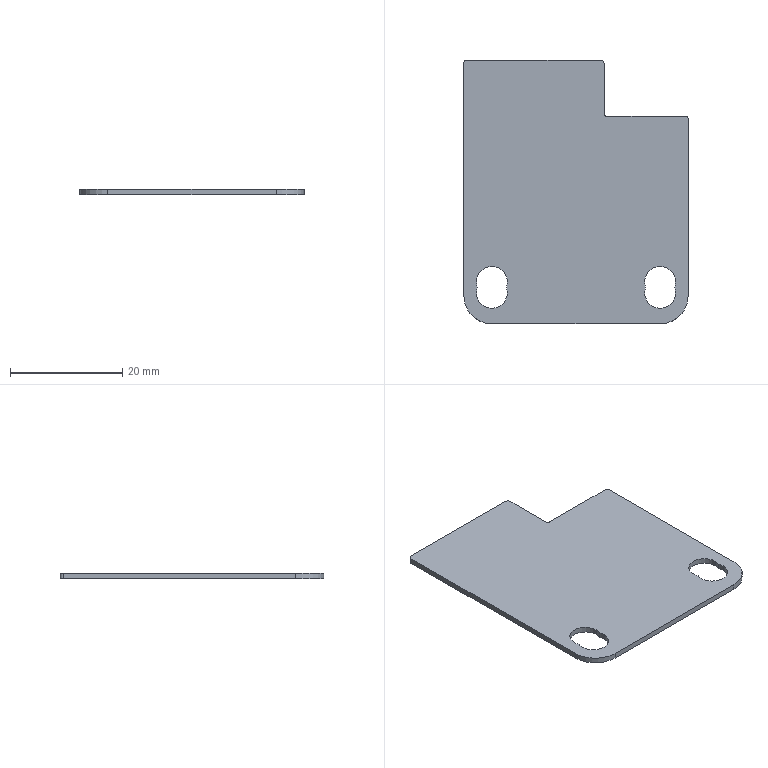Part | SolidWorks | features BaseBody 1 | 1 solid | 26 faces | box 40 x 47 x 1 mm | volume 1650 mm3 | cylinder 18 | plane 8 | commonest cylinder face diameters 5.5 x12 1 x4 10 x2
STEP:
#1=CARTESIAN_POINT('',(180.229,1870.544,-8.));
#2=VERTEX_POINT('',#1);
#3=CARTESIAN_POINT('',(180.041,1869.544,-8.));
#4=VERTEX_POINT('',#3);
#5=CARTESIAN_POINT('',(177.479,1870.544,-8.));
#6=DIRECTION('',(0.,0.,-1.));
#7=DIRECTION('',(-1.,0.,0.));
#8=AXIS2_PLACEMENT_3D('',#5,#6,#7);
#9=CIRCLE('',#8,2.75);
#10=EDGE_CURVE('',#2,#4,#9,.T.);
#11=ORIENTED_EDGE('',*,*,#10,.F.);
#12=CARTESIAN_POINT('',(180.229,1870.544,-9.));
#13=VERTEX_POINT('',#12);
#14=CARTESIAN_POINT('',(180.229,1870.544,-8.5));
#15=DIRECTION('',(0.,0.,-1.));
#16=VECTOR('',#15,1000.);
#17=LINE('',#14,#16);
#18=EDGE_CURVE('',#2,#13,#17,.T.);
#19=ORIENTED_EDGE('',*,*,#18,.T.);
#20=CARTESIAN_POINT('',(180.041,1869.544,-9.));
#21=VERTEX_POINT('',#20);
#22=CARTESIAN_POINT('',(177.479,1870.544,-9.));
#23=DIRECTION('',(0.,0.,1.));
#24=DIRECTION('',(-1.,0.,0.));
#25=AXIS2_PLACEMENT_3D('',#22,#23,#24);
#26=CIRCLE('',#25,2.75);
#27=EDGE_CURVE('',#21,#13,#26,.T.);
#28=ORIENTED_EDGE('',*,*,#27,.F.);
#29=CARTESIAN_POINT('',(180.041,1869.544,-8.5));
#30=DIRECTION('',(0.,0.,-1.));
#31=VECTOR('',#30,1000.);
#32=LINE('',#29,#31);
#33=EDGE_CURVE('',#4,#21,#32,.T.);
#34=ORIENTED_EDGE('',*,*,#33,.F.);
#35=EDGE_LOOP('',(#11,#19,#28,#34));
#36=FACE_OUTER_BOUND('',#35,.T.);
#37=CARTESIAN_POINT('',(177.479,1870.544,-8.5));
#38=DIRECTION('',(0.,0.,-1.));
#39=DIRECTION('',(-1.,0.,0.));
#40=AXIS2_PLACEMENT_3D('',#37,#38,#39);
#41=CYLINDRICAL_SURFACE('',#40,2.75);
#42=ADVANCED_FACE('',(#36),#41,.F.);
#43=ORIENTED_EDGE('',*,*,#18,.F.);
#44=CARTESIAN_POINT('',(174.729,1870.544,-8.));
#45=VERTEX_POINT('',#44);
#46=CARTESIAN_POINT('',(177.479,1870.544,-8.));
#47=DIRECTION('',(0.,0.,-1.));
#48=DIRECTION('',(-1.,0.,0.));
#49=AXIS2_PLACEMENT_3D('',#46,#47,#48);
#50=CIRCLE('',#49,2.75);
#51=EDGE_CURVE('',#45,#2,#50,.T.);
#52=ORIENTED_EDGE('',*,*,#51,.F.);
#53=CARTESIAN_POINT('',(174.729,1870.544,-9.));
#54=VERTEX_POINT('',#53);
#55=CARTESIAN_POINT('',(174.729,1870.544,-8.5));
#56=DIRECTION('',(0.,0.,-1.));
#57=VECTOR('',#56,1000.);
#58=LINE('',#55,#57);
#59=EDGE_CURVE('',#45,#54,#58,.T.);
#60=ORIENTED_EDGE('',*,*,#59,.T.);
#61=CARTESIAN_POINT('',(177.479,1870.544,-9.));
#62=DIRECTION('',(0.,0.,1.));
#63=DIRECTION('',(-1.,0.,0.));
#64=AXIS2_PLACEMENT_3D('',#61,#62,#63);
#65=CIRCLE('',#64,2.75);
#66=EDGE_CURVE('',#13,#54,#65,.T.);
#67=ORIENTED_EDGE('',*,*,#66,.F.);
#68=EDGE_LOOP('',(#43,#52,#60,#67));
#69=FACE_OUTER_BOUND('',#68,.T.);
#70=CARTESIAN_POINT('',(177.479,1870.544,-8.5));
#71=DIRECTION('',(0.,0.,-1.));
#72=DIRECTION('',(-1.,0.,0.));
#73=AXIS2_PLACEMENT_3D('',#70,#71,#72);
#74=CYLINDRICAL_SURFACE('',#73,2.75);
#75=ADVANCED_FACE('',(#69),#74,.F.);
#76=CARTESIAN_POINT('',(180.229,1868.544,-8.));
#77=VERTEX_POINT('',#76);
#78=CARTESIAN_POINT('',(174.729,1868.544,-8.));
#79=VERTEX_POINT('',#78);
#80=CARTESIAN_POINT('',(177.479,1868.544,-8.));
#81=DIRECTION('',(0.,0.,-1.));
#82=DIRECTION('',(-1.,0.,0.));
#83=AXIS2_PLACEMENT_3D('',#80,#81,#82);
#84=CIRCLE('',#83,2.75);
#85=EDGE_CURVE('',#77,#79,#84,.T.);
#86=ORIENTED_EDGE('',*,*,#85,.F.);
#87=CARTESIAN_POINT('',(180.229,1868.544,-9.));
#88=VERTEX_POINT('',#87);
#89=CARTESIAN_POINT('',(180.229,1868.544,-8.5));
#90=DIRECTION('',(0.,0.,-1.));
#91=VECTOR('',#90,1000.);
#92=LINE('',#89,#91);
#93=EDGE_CURVE('',#77,#88,#92,.T.);
#94=ORIENTED_EDGE('',*,*,#93,.T.);
#95=CARTESIAN_POINT('',(174.729,1868.544,-9.));
#96=VERTEX_POINT('',#95);
#97=CARTESIAN_POINT('',(177.479,1868.544,-9.));
#98=DIRECTION('',(0.,0.,1.));
#99=DIRECTION('',(-1.,0.,0.));
#100=AXIS2_PLACEMENT_3D('',#97,#98,#99);
#101=CIRCLE('',#100,2.75);
#102=EDGE_CURVE('',#96,#88,#101,.T.);
#103=ORIENTED_EDGE('',*,*,#102,.F.);
#104=CARTESIAN_POINT('',(174.729,1868.544,-8.5));
#105=DIRECTION('',(0.,0.,-1.));
#106=VECTOR('',#105,1000.);
#107=LINE('',#104,#106);
#108=EDGE_CURVE('',#79,#96,#107,.T.);
#109=ORIENTED_EDGE('',*,*,#108,.F.);
#110=EDGE_LOOP('',(#86,#94,#103,#109));
#111=FACE_OUTER_BOUND('',#110,.T.);
#112=CARTESIAN_POINT('',(177.479,1868.544,-8.5));
#113=DIRECTION('',(0.,0.,-1.));
#114=DIRECTION('',(-1.,0.,0.));
#115=AXIS2_PLACEMENT_3D('',#112,#113,#114);
#116=CYLINDRICAL_SURFACE('',#115,2.75);
#117=ADVANCED_FACE('',(#111),#116,.F.);
#118=CARTESIAN_POINT('',(174.917,1869.544,-8.));
#119=VERTEX_POINT('',#118);
#120=CARTESIAN_POINT('',(177.479,1868.544,-8.));
#121=DIRECTION('',(0.,0.,-1.));
#122=DIRECTION('',(-1.,0.,0.));
#123=AXIS2_PLACEMENT_3D('',#120,#121,#122);
#124=CIRCLE('',#123,2.75);
#125=EDGE_CURVE('',#79,#119,#124,.T.);
#126=ORIENTED_EDGE('',*,*,#125,.F.);
#127=ORIENTED_EDGE('',*,*,#108,.T.);
#128=CARTESIAN_POINT('',(174.917,1869.544,-9.));
#129=VERTEX_POINT('',#128);
#130=CARTESIAN_POINT('',(177.479,1868.544,-9.));
#131=DIRECTION('',(0.,0.,1.));
#132=DIRECTION('',(-1.,0.,0.));
#133=AXIS2_PLACEMENT_3D('',#130,#131,#132);
#134=CIRCLE('',#133,2.75);
#135=EDGE_CURVE('',#129,#96,#134,.T.);
#136=ORIENTED_EDGE('',*,*,#135,.F.);
#137=CARTESIAN_POINT('',(174.917,1869.544,-8.5));
#138=DIRECTION('',(0.,0.,1.));
#139=VECTOR('',#138,1000.);
#140=LINE('',#137,#139);
#141=EDGE_CURVE('',#129,#119,#140,.T.);
#142=ORIENTED_EDGE('',*,*,#141,.T.);
#143=EDGE_LOOP('',(#126,#127,#136,#142));
#144=FACE_OUTER_BOUND('',#143,.T.);
#145=CARTESIAN_POINT('',(177.479,1868.544,-8.5));
#146=DIRECTION('',(0.,0.,-1.));
#147=DIRECTION('',(-1.,0.,0.));
#148=AXIS2_PLACEMENT_3D('',#145,#146,#147);
#149=CYLINDRICAL_SURFACE('',#148,2.75);
#150=ADVANCED_FACE('',(#144),#149,.F.);
#151=CARTESIAN_POINT('',(204.729,1870.544,-9.));
#152=VERTEX_POINT('',#151);
#153=CARTESIAN_POINT('',(204.917,1869.544,-9.));
#154=VERTEX_POINT('',#153);
#155=CARTESIAN_POINT('',(207.479,1870.544,-9.));
#156=DIRECTION('',(0.,0.,1.));
#157=DIRECTION('',(1.,0.,0.));
#158=AXIS2_PLACEMENT_3D('',#155,#156,#157);
#159=CIRCLE('',#158,2.75);
#160=EDGE_CURVE('',#152,#154,#159,.T.);
#161=ORIENTED_EDGE('',*,*,#160,.F.);
#162=CARTESIAN_POINT('',(204.729,1870.544,-8.));
#163=VERTEX_POINT('',#162);
#164=CARTESIAN_POINT('',(204.729,1870.544,-8.5));
#165=DIRECTION('',(0.,0.,1.));
#166=VECTOR('',#165,1000.);
#167=LINE('',#164,#166);
#168=EDGE_CURVE('',#152,#163,#167,.T.);
#169=ORIENTED_EDGE('',*,*,#168,.T.);
#170=CARTESIAN_POINT('',(204.917,1869.544,-8.));
#171=VERTEX_POINT('',#170);
#172=CARTESIAN_POINT('',(207.479,1870.544,-8.));
#173=DIRECTION('',(0.,0.,-1.));
#174=DIRECTION('',(1.,0.,0.));
#175=AXIS2_PLACEMENT_3D('',#172,#173,#174);
#176=CIRCLE('',#175,2.75);
#177=EDGE_CURVE('',#171,#163,#176,.T.);
#178=ORIENTED_EDGE('',*,*,#177,.F.);
#179=CARTESIAN_POINT('',(204.917,1869.544,-8.5));
#180=DIRECTION('',(0.,0.,1.));
#181=VECTOR('',#180,1000.);
#182=LINE('',#179,#181);
#183=EDGE_CURVE('',#154,#171,#182,.T.);
#184=ORIENTED_EDGE('',*,*,#183,.F.);
#185=EDGE_LOOP('',(#161,#169,#178,#184));
#186=FACE_OUTER_BOUND('',#185,.T.);
#187=CARTESIAN_POINT('',(207.479,1870.544,-8.5));
#188=DIRECTION('',(0.,0.,1.));
#189=DIRECTION('',(1.,0.,0.));
#190=AXIS2_PLACEMENT_3D('',#187,#188,#189);
#191=CYLINDRICAL_SURFACE('',#190,2.75);
#192=ADVANCED_FACE('',(#186),#191,.F.);
#193=ORIENTED_EDGE('',*,*,#168,.F.);
#194=CARTESIAN_POINT('',(210.229,1870.544,-9.));
#195=VERTEX_POINT('',#194);
#196=CARTESIAN_POINT('',(207.479,1870.544,-9.));
#197=DIRECTION('',(0.,0.,1.));
#198=DIRECTION('',(1.,0.,0.));
#199=AXIS2_PLACEMENT_3D('',#196,#197,#198);
#200=CIRCLE('',#199,2.75);
#201=EDGE_CURVE('',#195,#152,#200,.T.);
#202=ORIENTED_EDGE('',*,*,#201,.F.);
#203=CARTESIAN_POINT('',(210.229,1870.544,-8.));
#204=VERTEX_POINT('',#203);
#205=CARTESIAN_POINT('',(210.229,1870.544,-8.5));
#206=DIRECTION('',(0.,0.,1.));
#207=VECTOR('',#206,1000.);
#208=LINE('',#205,#207);
#209=EDGE_CURVE('',#195,#204,#208,.T.);
#210=ORIENTED_EDGE('',*,*,#209,.T.);
#211=CARTESIAN_POINT('',(207.479,1870.544,-8.));
#212=DIRECTION('',(0.,0.,-1.));
#213=DIRECTION('',(1.,0.,0.));
#214=AXIS2_PLACEMENT_3D('',#211,#212,#213);
#215=CIRCLE('',#214,2.75);
#216=EDGE_CURVE('',#163,#204,#215,.T.);
#217=ORIENTED_EDGE('',*,*,#216,.F.);
#218=EDGE_LOOP('',(#193,#202,#210,#217));
#219=FACE_OUTER_BOUND('',#218,.T.);
#220=CARTESIAN_POINT('',(207.479,1870.544,-8.5));
#221=DIRECTION('',(0.,0.,1.));
#222=DIRECTION('',(1.,0.,0.));
#223=AXIS2_PLACEMENT_3D('',#220,#221,#222);
#224=CYLINDRICAL_SURFACE('',#223,2.75);
#225=ADVANCED_FACE('',(#219),#224,.F.);
#226=CARTESIAN_POINT('',(204.729,1868.544,-9.));
#227=VERTEX_POINT('',#226);
#228=CARTESIAN_POINT('',(210.229,1868.544,-9.));
#229=VERTEX_POINT('',#228);
#230=CARTESIAN_POINT('',(207.479,1868.544,-9.));
#231=DIRECTION('',(0.,0.,1.));
#232=DIRECTION('',(1.,0.,0.));
#233=AXIS2_PLACEMENT_3D('',#230,#231,#232);
#234=CIRCLE('',#233,2.75);
#235=EDGE_CURVE('',#227,#229,#234,.T.);
#236=ORIENTED_EDGE('',*,*,#235,.F.);
#237=CARTESIAN_POINT('',(204.729,1868.544,-8.));
#238=VERTEX_POINT('',#237);
#239=CARTESIAN_POINT('',(204.729,1868.544,-8.5));
#240=DIRECTION('',(0.,0.,1.));
#241=VECTOR('',#240,1000.);
#242=LINE('',#239,#241);
#243=EDGE_CURVE('',#227,#238,#242,.T.);
#244=ORIENTED_EDGE('',*,*,#243,.T.);
#245=CARTESIAN_POINT('',(210.229,1868.544,-8.));
#246=VERTEX_POINT('',#245);
#247=CARTESIAN_POINT('',(207.479,1868.544,-8.));
#248=DIRECTION('',(0.,0.,-1.));
#249=DIRECTION('',(1.,0.,0.));
#250=AXIS2_PLACEMENT_3D('',#247,#248,#249);
#251=CIRCLE('',#250,2.75);
#252=EDGE_CURVE('',#246,#238,#251,.T.);
#253=ORIENTED_EDGE('',*,*,#252,.F.);
#254=CARTESIAN_POINT('',(210.229,1868.544,-8.5));
#255=DIRECTION('',(0.,0.,1.));
#256=VECTOR('',#255,1000.);
#257=LINE('',#254,#256);
#258=EDGE_CURVE('',#229,#246,#257,.T.);
#259=ORIENTED_EDGE('',*,*,#258,.F.);
#260=EDGE_LOOP('',(#236,#244,#253,#259));
#261=FACE_OUTER_BOUND('',#260,.T.);
#262=CARTESIAN_POINT('',(207.479,1868.544,-8.5));
#263=DIRECTION('',(0.,0.,1.));
#264=DIRECTION('',(1.,0.,0.));
#265=AXIS2_PLACEMENT_3D('',#262,#263,#264);
#266=CYLINDRICAL_SURFACE('',#265,2.75);
#267=ADVANCED_FACE('',(#261),#266,.F.);
#268=CARTESIAN_POINT('',(210.041,1869.544,-9.));
#269=VERTEX_POINT('',#268);
#270=CARTESIAN_POINT('',(207.479,1868.544,-9.));
#271=DIRECTION('',(0.,0.,1.));
#272=DIRECTION('',(1.,0.,0.));
#273=AXIS2_PLACEMENT_3D('',#270,#271,#272);
#274=CIRCLE('',#273,2.75);
#275=EDGE_CURVE('',#229,#269,#274,.T.);
#276=ORIENTED_EDGE('',*,*,#275,.F.);
#277=ORIENTED_EDGE('',*,*,#258,.T.);
#278=CARTESIAN_POINT('',(210.041,1869.544,-8.));
#279=VERTEX_POINT('',#278);
#280=CARTESIAN_POINT('',(207.479,1868.544,-8.));
#281=DIRECTION('',(0.,0.,-1.));
#282=DIRECTION('',(1.,0.,0.));
#283=AXIS2_PLACEMENT_3D('',#280,#281,#282);
#284=CIRCLE('',#283,2.75);
#285=EDGE_CURVE('',#279,#246,#284,.T.);
#286=ORIENTED_EDGE('',*,*,#285,.F.);
#287=CARTESIAN_POINT('',(210.041,1869.544,-8.5));
#288=DIRECTION('',(0.,0.,-1.));
#289=VECTOR('',#288,1000.);
#290=LINE('',#287,#289);
#291=EDGE_CURVE('',#279,#269,#290,.T.);
#292=ORIENTED_EDGE('',*,*,#291,.T.);
#293=EDGE_LOOP('',(#276,#277,#286,#292));
#294=FACE_OUTER_BOUND('',#293,.T.);
#295=CARTESIAN_POINT('',(207.479,1868.544,-8.5));
#296=DIRECTION('',(0.,0.,1.));
#297=DIRECTION('',(1.,0.,0.));
#298=AXIS2_PLACEMENT_3D('',#295,#296,#297);
#299=CYLINDRICAL_SURFACE('',#298,2.75);
#300=ADVANCED_FACE('',(#294),#299,.F.);
#301=CARTESIAN_POINT('',(177.479,1868.544,-8.));
#302=DIRECTION('',(0.,0.,-1.));
#303=DIRECTION('',(-1.,0.,0.));
#304=AXIS2_PLACEMENT_3D('',#301,#302,#303);
#305=CIRCLE('',#304,2.75);
#306=EDGE_CURVE('',#4,#77,#305,.T.);
#307=ORIENTED_EDGE('',*,*,#306,.T.);
#308=ORIENTED_EDGE('',*,*,#85,.T.);
#309=ORIENTED_EDGE('',*,*,#125,.T.);
#310=CARTESIAN_POINT('',(177.479,1870.544,-8.));
#311=DIRECTION('',(0.,0.,-1.));
#312=DIRECTION('',(-1.,0.,0.));
#313=AXIS2_PLACEMENT_3D('',#310,#311,#312);
#314=CIRCLE('',#313,2.75);
#315=EDGE_CURVE('',#119,#45,#314,.T.);
#316=ORIENTED_EDGE('',*,*,#315,.T.);
#317=ORIENTED_EDGE('',*,*,#51,.T.);
#318=ORIENTED_EDGE('',*,*,#10,.T.);
#319=EDGE_LOOP('',(#307,#308,#309,#316,#317,#318));
#320=FACE_BOUND('',#319,.T.);
#321=ORIENTED_EDGE('',*,*,#285,.T.);
#322=ORIENTED_EDGE('',*,*,#252,.T.);
#323=CARTESIAN_POINT('',(207.479,1868.544,-8.));
#324=DIRECTION('',(0.,0.,-1.));
#325=DIRECTION('',(1.,0.,0.));
#326=AXIS2_PLACEMENT_3D('',#323,#324,#325);
#327=CIRCLE('',#326,2.75);
#328=EDGE_CURVE('',#238,#171,#327,.T.);
#329=ORIENTED_EDGE('',*,*,#328,.T.);
#330=ORIENTED_EDGE('',*,*,#177,.T.);
#331=ORIENTED_EDGE('',*,*,#216,.T.);
#332=CARTESIAN_POINT('',(207.479,1870.544,-8.));
#333=DIRECTION('',(0.,0.,-1.));
#334=DIRECTION('',(1.,0.,0.));
#335=AXIS2_PLACEMENT_3D('',#332,#333,#334);
#336=CIRCLE('',#335,2.75);
#337=EDGE_CURVE('',#204,#279,#336,.T.);
#338=ORIENTED_EDGE('',*,*,#337,.T.);
#339=EDGE_LOOP('',(#321,#322,#329,#330,#331,#338));
#340=FACE_BOUND('',#339,.T.);
#341=CARTESIAN_POINT('',(211.979,1900.044,-8.));
#342=VERTEX_POINT('',#341);
#343=CARTESIAN_POINT('',(197.979,1900.044,-8.));
#344=VERTEX_POINT('',#343);
#345=CARTESIAN_POINT('',(192.479,1900.044,-8.));
#346=DIRECTION('',(-1.,0.,0.));
#347=VECTOR('',#346,1000.);
#348=LINE('',#345,#347);
#349=EDGE_CURVE('',#342,#344,#348,.T.);
#350=ORIENTED_EDGE('',*,*,#349,.T.);
#351=CARTESIAN_POINT('',(197.479,1900.544,-8.));
#352=VERTEX_POINT('',#351);
#353=CARTESIAN_POINT('',(197.979,1900.544,-8.));
#354=DIRECTION('',(0.,0.,-1.));
#355=DIRECTION('',(-1.,0.,0.));
#356=AXIS2_PLACEMENT_3D('',#353,#354,#355);
#357=CIRCLE('',#356,0.5);
#358=EDGE_CURVE('',#344,#352,#357,.T.);
#359=ORIENTED_EDGE('',*,*,#358,.T.);
#360=CARTESIAN_POINT('',(197.479,1909.544,-8.));
#361=VERTEX_POINT('',#360);
#362=CARTESIAN_POINT('',(197.479,1886.544,-8.));
#363=DIRECTION('',(0.,1.,0.));
#364=VECTOR('',#363,1000.);
#365=LINE('',#362,#364);
#366=EDGE_CURVE('',#352,#361,#365,.T.);
#367=ORIENTED_EDGE('',*,*,#366,.T.);
#368=CARTESIAN_POINT('',(196.979,1910.044,-8.));
#369=VERTEX_POINT('',#368);
#370=CARTESIAN_POINT('',(196.979,1909.544,-8.));
#371=DIRECTION('',(0.,0.,1.));
#372=DIRECTION('',(-1.,0.,0.));
#373=AXIS2_PLACEMENT_3D('',#370,#371,#372);
#374=CIRCLE('',#373,0.5);
#375=EDGE_CURVE('',#361,#369,#374,.T.);
#376=ORIENTED_EDGE('',*,*,#375,.T.);
#377=CARTESIAN_POINT('',(172.979,1910.044,-8.));
#378=VERTEX_POINT('',#377);
#379=CARTESIAN_POINT('',(192.479,1910.044,-8.));
#380=DIRECTION('',(-1.,0.,0.));
#381=VECTOR('',#380,1000.);
#382=LINE('',#379,#381);
#383=EDGE_CURVE('',#369,#378,#382,.T.);
#384=ORIENTED_EDGE('',*,*,#383,.T.);
#385=CARTESIAN_POINT('',(172.479,1909.544,-8.));
#386=VERTEX_POINT('',#385);
#387=CARTESIAN_POINT('',(172.979,1909.544,-8.));
#388=DIRECTION('',(0.,0.,1.));
#389=DIRECTION('',(1.,0.,0.));
#390=AXIS2_PLACEMENT_3D('',#387,#388,#389);
#391=CIRCLE('',#390,0.5);
#392=EDGE_CURVE('',#378,#386,#391,.T.);
#393=ORIENTED_EDGE('',*,*,#392,.T.);
#394=CARTESIAN_POINT('',(172.479,1868.044,-8.));
#395=VERTEX_POINT('',#394);
#396=CARTESIAN_POINT('',(172.479,1886.544,-8.));
#397=DIRECTION('',(0.,-1.,0.));
#398=VECTOR('',#397,1000.);
#399=LINE('',#396,#398);
#400=EDGE_CURVE('',#386,#395,#399,.T.);
#401=ORIENTED_EDGE('',*,*,#400,.T.);
#402=CARTESIAN_POINT('',(177.479,1863.044,-8.));
#403=VERTEX_POINT('',#402);
#404=CARTESIAN_POINT('',(177.479,1868.044,-8.));
#405=DIRECTION('',(0.,0.,1.));
#406=DIRECTION('',(1.,0.,0.));
#407=AXIS2_PLACEMENT_3D('',#404,#405,#406);
#408=CIRCLE('',#407,5.);
#409=EDGE_CURVE('',#395,#403,#408,.T.);
#410=ORIENTED_EDGE('',*,*,#409,.T.);
#411=CARTESIAN_POINT('',(207.479,1863.044,-8.));
#412=VERTEX_POINT('',#411);
#413=CARTESIAN_POINT('',(192.479,1863.044,-8.));
#414=DIRECTION('',(1.,0.,0.));
#415=VECTOR('',#414,1000.);
#416=LINE('',#413,#415);
#417=EDGE_CURVE('',#403,#412,#416,.T.);
#418=ORIENTED_EDGE('',*,*,#417,.T.);
#419=CARTESIAN_POINT('',(212.479,1868.044,-8.));
#420=VERTEX_POINT('',#419);
#421=CARTESIAN_POINT('',(207.479,1868.044,-8.));
#422=DIRECTION('',(0.,0.,1.));
#423=DIRECTION('',(1.,0.,0.));
#424=AXIS2_PLACEMENT_3D('',#421,#422,#423);
#425=CIRCLE('',#424,5.);
#426=EDGE_CURVE('',#412,#420,#425,.T.);
#427=ORIENTED_EDGE('',*,*,#426,.T.);
#428=CARTESIAN_POINT('',(212.479,1899.544,-8.));
#429=VERTEX_POINT('',#428);
#430=CARTESIAN_POINT('',(212.479,1886.544,-8.));
#431=DIRECTION('',(0.,1.,0.));
#432=VECTOR('',#431,1000.);
#433=LINE('',#430,#432);
#434=EDGE_CURVE('',#420,#429,#433,.T.);
#435=ORIENTED_EDGE('',*,*,#434,.T.);
#436=CARTESIAN_POINT('',(211.979,1899.544,-8.));
#437=DIRECTION('',(0.,0.,1.));
#438=DIRECTION('',(1.,0.,0.));
#439=AXIS2_PLACEMENT_3D('',#436,#437,#438);
#440=CIRCLE('',#439,0.5);
#441=EDGE_CURVE('',#429,#342,#440,.T.);
#442=ORIENTED_EDGE('',*,*,#441,.T.);
#443=EDGE_LOOP('',(#350,#359,#367,#376,#384,#393,#401,#410,#418,#427,#435,#442));
#444=FACE_OUTER_BOUND('',#443,.T.);
#445=CARTESIAN_POINT('',(192.479,1886.544,-8.));
#446=DIRECTION('',(0.,0.,1.));
#447=DIRECTION('',(1.,0.,0.));
#448=AXIS2_PLACEMENT_3D('',#445,#446,#447);
#449=PLANE('',#448);
#450=ADVANCED_FACE('',(#320,#340,#444),#449,.T.);
#451=ORIENTED_EDGE('',*,*,#59,.F.);
#452=ORIENTED_EDGE('',*,*,#315,.F.);
#453=ORIENTED_EDGE('',*,*,#141,.F.);
#454=CARTESIAN_POINT('',(177.479,1870.544,-9.));
#455=DIRECTION('',(0.,0.,1.));
#456=DIRECTION('',(-1.,0.,0.));
#457=AXIS2_PLACEMENT_3D('',#454,#455,#456);
#458=CIRCLE('',#457,2.75);
#459=EDGE_CURVE('',#54,#129,#458,.T.);
#460=ORIENTED_EDGE('',*,*,#459,.F.);
#461=EDGE_LOOP('',(#451,#452,#453,#460));
#462=FACE_OUTER_BOUND('',#461,.T.);
#463=CARTESIAN_POINT('',(177.479,1870.544,-8.5));
#464=DIRECTION('',(0.,0.,-1.));
#465=DIRECTION('',(-1.,0.,0.));
#466=AXIS2_PLACEMENT_3D('',#463,#464,#465);
#467=CYLINDRICAL_SURFACE('',#466,2.75);
#468=ADVANCED_FACE('',(#462),#467,.F.);
#469=ORIENTED_EDGE('',*,*,#93,.F.);
#470=ORIENTED_EDGE('',*,*,#306,.F.);
#471=ORIENTED_EDGE('',*,*,#33,.T.);
#472=CARTESIAN_POINT('',(177.479,1868.544,-9.));
#473=DIRECTION('',(0.,0.,1.));
#474=DIRECTION('',(-1.,0.,0.));
#475=AXIS2_PLACEMENT_3D('',#472,#473,#474);
#476=CIRCLE('',#475,2.75);
#477=EDGE_CURVE('',#88,#21,#476,.T.);
#478=ORIENTED_EDGE('',*,*,#477,.F.);
#479=EDGE_LOOP('',(#469,#470,#471,#478));
#480=FACE_OUTER_BOUND('',#479,.T.);
#481=CARTESIAN_POINT('',(177.479,1868.544,-8.5));
#482=DIRECTION('',(0.,0.,-1.));
#483=DIRECTION('',(-1.,0.,0.));
#484=AXIS2_PLACEMENT_3D('',#481,#482,#483);
#485=CYLINDRICAL_SURFACE('',#484,2.75);
#486=ADVANCED_FACE('',(#480),#485,.F.);
#487=ORIENTED_EDGE('',*,*,#209,.F.);
#488=CARTESIAN_POINT('',(207.479,1870.544,-9.));
#489=DIRECTION('',(0.,0.,1.));
#490=DIRECTION('',(1.,0.,0.));
#491=AXIS2_PLACEMENT_3D('',#488,#489,#490);
#492=CIRCLE('',#491,2.75);
#493=EDGE_CURVE('',#269,#195,#492,.T.);
#494=ORIENTED_EDGE('',*,*,#493,.F.);
#495=ORIENTED_EDGE('',*,*,#291,.F.);
#496=ORIENTED_EDGE('',*,*,#337,.F.);
#497=EDGE_LOOP('',(#487,#494,#495,#496));
#498=FACE_OUTER_BOUND('',#497,.T.);
#499=CARTESIAN_POINT('',(207.479,1870.544,-8.5));
#500=DIRECTION('',(0.,0.,1.));
#501=DIRECTION('',(1.,0.,0.));
#502=AXIS2_PLACEMENT_3D('',#499,#500,#501);
#503=CYLINDRICAL_SURFACE('',#502,2.75);
#504=ADVANCED_FACE('',(#498),#503,.F.);
#505=ORIENTED_EDGE('',*,*,#243,.F.);
#506=CARTESIAN_POINT('',(207.479,1868.544,-9.));
#507=DIRECTION('',(0.,0.,1.));
#508=DIRECTION('',(1.,0.,0.));
#509=AXIS2_PLACEMENT_3D('',#506,#507,#508);
#510=CIRCLE('',#509,2.75);
#511=EDGE_CURVE('',#154,#227,#510,.T.);
#512=ORIENTED_EDGE('',*,*,#511,.F.);
#513=ORIENTED_EDGE('',*,*,#183,.T.);
#514=ORIENTED_EDGE('',*,*,#328,.F.);
#515=EDGE_LOOP('',(#505,#512,#513,#514));
#516=FACE_OUTER_BOUND('',#515,.T.);
#517=CARTESIAN_POINT('',(207.479,1868.544,-8.5));
#518=DIRECTION('',(0.,0.,1.));
#519=DIRECTION('',(1.,0.,0.));
#520=AXIS2_PLACEMENT_3D('',#517,#518,#519);
#521=CYLINDRICAL_SURFACE('',#520,2.75);
#522=ADVANCED_FACE('',(#516),#521,.F.);
#523=CARTESIAN_POINT('',(197.479,1900.544,-9.));
#524=VERTEX_POINT('',#523);
#525=CARTESIAN_POINT('',(197.479,1900.544,-8.));
#526=DIRECTION('',(0.,0.,-1.));
#527=VECTOR('',#526,1000.);
#528=LINE('',#525,#527);
#529=EDGE_CURVE('',#352,#524,#528,.T.);
#530=ORIENTED_EDGE('',*,*,#529,.F.);
#531=ORIENTED_EDGE('',*,*,#358,.F.);
#532=CARTESIAN_POINT('',(197.979,1900.044,-9.));
#533=VERTEX_POINT('',#532);
#534=CARTESIAN_POINT('',(197.979,1900.044,-8.));
#535=DIRECTION('',(0.,0.,1.));
#536=VECTOR('',#535,1000.);
#537=LINE('',#534,#536);
#538=EDGE_CURVE('',#533,#344,#537,.T.);
#539=ORIENTED_EDGE('',*,*,#538,.F.);
#540=CARTESIAN_POINT('',(197.979,1900.544,-9.));
#541=DIRECTION('',(0.,0.,1.));
#542=DIRECTION('',(-1.,0.,0.));
#543=AXIS2_PLACEMENT_3D('',#540,#541,#542);
#544=CIRCLE('',#543,0.5);
#545=EDGE_CURVE('',#524,#533,#544,.T.);
#546=ORIENTED_EDGE('',*,*,#545,.F.);
#547=EDGE_LOOP('',(#530,#531,#539,#546));
#548=FACE_OUTER_BOUND('',#547,.T.);
#549=CARTESIAN_POINT('',(197.979,1900.544,-8.));
#550=DIRECTION('',(0.,0.,-1.));
#551=DIRECTION('',(-1.,0.,0.));
#552=AXIS2_PLACEMENT_3D('',#549,#550,#551);
#553=CYLINDRICAL_SURFACE('',#552,0.5);
#554=ADVANCED_FACE('',(#548),#553,.F.);
#555=CARTESIAN_POINT('',(211.979,1900.044,-9.));
#556=VERTEX_POINT('',#555);
#557=CARTESIAN_POINT('',(197.479,1900.044,-9.));
#558=DIRECTION('',(1.,0.,0.));
#559=VECTOR('',#558,1000.);
#560=LINE('',#557,#559);
#561=EDGE_CURVE('',#533,#556,#560,.T.);
#562=ORIENTED_EDGE('',*,*,#561,.F.);
#563=ORIENTED_EDGE('',*,*,#538,.T.);
#564=ORIENTED_EDGE('',*,*,#349,.F.);
#565=CARTESIAN_POINT('',(211.979,1900.044,-8.));
#566=DIRECTION('',(0.,0.,1.));
#567=VECTOR('',#566,1000.);
#568=LINE('',#565,#567);
#569=EDGE_CURVE('',#556,#342,#568,.T.);
#570=ORIENTED_EDGE('',*,*,#569,.F.);
#571=EDGE_LOOP('',(#562,#563,#564,#570));
#572=FACE_OUTER_BOUND('',#571,.T.);
#573=CARTESIAN_POINT('',(197.479,1900.044,-8.));
#574=DIRECTION('',(0.,-1.,0.));
#575=DIRECTION('',(0.,0.,-1.));
#576=AXIS2_PLACEMENT_3D('',#573,#574,#575);
#577=PLANE('',#576);
#578=ADVANCED_FACE('',(#572),#577,.F.);
#579=CARTESIAN_POINT('',(212.479,1899.544,-9.));
#580=VERTEX_POINT('',#579);
#581=CARTESIAN_POINT('',(212.479,1899.544,-8.5));
#582=DIRECTION('',(0.,0.,-1.));
#583=VECTOR('',#582,1000.);
#584=LINE('',#581,#583);
#585=EDGE_CURVE('',#429,#580,#584,.T.);
#586=ORIENTED_EDGE('',*,*,#585,.T.);
#587=CARTESIAN_POINT('',(211.979,1899.544,-9.));
#588=DIRECTION('',(0.,0.,1.));
#589=DIRECTION('',(1.,0.,0.));
#590=AXIS2_PLACEMENT_3D('',#587,#588,#589);
#591=CIRCLE('',#590,0.5);
#592=EDGE_CURVE('',#580,#556,#591,.T.);
#593=ORIENTED_EDGE('',*,*,#592,.T.);
#594=ORIENTED_EDGE('',*,*,#569,.T.);
#595=ORIENTED_EDGE('',*,*,#441,.F.);
#596=EDGE_LOOP('',(#586,#593,#594,#595));
#597=FACE_OUTER_BOUND('',#596,.T.);
#598=CARTESIAN_POINT('',(211.979,1899.544,-8.5));
#599=DIRECTION('',(0.,0.,1.));
#600=DIRECTION('',(1.,0.,0.));
#601=AXIS2_PLACEMENT_3D('',#598,#599,#600);
#602=CYLINDRICAL_SURFACE('',#601,0.5);
#603=ADVANCED_FACE('',(#597),#602,.T.);
#604=ORIENTED_EDGE('',*,*,#434,.F.);
#605=CARTESIAN_POINT('',(212.479,1868.044,-9.));
#606=VERTEX_POINT('',#605);
#607=CARTESIAN_POINT('',(212.479,1868.044,-9.));
#608=DIRECTION('',(0.,0.,-1.));
#609=VECTOR('',#608,1000.);
#610=LINE('',#607,#609);
#611=EDGE_CURVE('',#420,#606,#610,.T.);
#612=ORIENTED_EDGE('',*,*,#611,.T.);
#613=CARTESIAN_POINT('',(212.479,1910.044,-9.));
#614=DIRECTION('',(0.,1.,0.));
#615=VECTOR('',#614,1000.);
#616=LINE('',#613,#615);
#617=EDGE_CURVE('',#606,#580,#616,.T.);
#618=ORIENTED_EDGE('',*,*,#617,.T.);
#619=ORIENTED_EDGE('',*,*,#585,.F.);
#620=EDGE_LOOP('',(#604,#612,#618,#619));
#621=FACE_OUTER_BOUND('',#620,.T.);
#622=CARTESIAN_POINT('',(212.479,1910.044,-9.));
#623=DIRECTION('',(1.,0.,0.));
#624=DIRECTION('',(0.,0.,-1.));
#625=AXIS2_PLACEMENT_3D('',#622,#623,#624);
#626=PLANE('',#625);
#627=ADVANCED_FACE('',(#621),#626,.T.);
#628=CARTESIAN_POINT('',(207.479,1863.044,-9.));
#629=VERTEX_POINT('',#628);
#630=CARTESIAN_POINT('',(207.479,1863.044,-9.));
#631=DIRECTION('',(0.,0.,-1.));
#632=VECTOR('',#631,1000.);
#633=LINE('',#630,#632);
#634=EDGE_CURVE('',#412,#629,#633,.T.);
#635=ORIENTED_EDGE('',*,*,#634,.T.);
#636=CARTESIAN_POINT('',(207.479,1868.044,-9.));
#637=DIRECTION('',(0.,0.,1.));
#638=DIRECTION('',(1.,0.,0.));
#639=AXIS2_PLACEMENT_3D('',#636,#637,#638);
#640=CIRCLE('',#639,5.);
#641=EDGE_CURVE('',#629,#606,#640,.T.);
#642=ORIENTED_EDGE('',*,*,#641,.T.);
#643=ORIENTED_EDGE('',*,*,#611,.F.);
#644=ORIENTED_EDGE('',*,*,#426,.F.);
#645=EDGE_LOOP('',(#635,#642,#643,#644));
#646=FACE_OUTER_BOUND('',#645,.T.);
#647=CARTESIAN_POINT('',(207.479,1868.044,-9.));
#648=DIRECTION('',(0.,0.,1.));
#649=DIRECTION('',(1.,0.,0.));
#650=AXIS2_PLACEMENT_3D('',#647,#648,#649);
#651=CYLINDRICAL_SURFACE('',#650,5.);
#652=ADVANCED_FACE('',(#646),#651,.T.);
#653=CARTESIAN_POINT('',(177.479,1863.044,-9.));
#654=VERTEX_POINT('',#653);
#655=CARTESIAN_POINT('',(212.479,1863.044,-9.));
#656=DIRECTION('',(1.,0.,0.));
#657=VECTOR('',#656,1000.);
#658=LINE('',#655,#657);
#659=EDGE_CURVE('',#654,#629,#658,.T.);
#660=ORIENTED_EDGE('',*,*,#659,.T.);
#661=ORIENTED_EDGE('',*,*,#634,.F.);
#662=ORIENTED_EDGE('',*,*,#417,.F.);
#663=CARTESIAN_POINT('',(177.479,1863.044,-9.));
#664=DIRECTION('',(0.,0.,-1.));
#665=VECTOR('',#664,1000.);
#666=LINE('',#663,#665);
#667=EDGE_CURVE('',#403,#654,#666,.T.);
#668=ORIENTED_EDGE('',*,*,#667,.T.);
#669=EDGE_LOOP('',(#660,#661,#662,#668));
#670=FACE_OUTER_BOUND('',#669,.T.);
#671=CARTESIAN_POINT('',(212.479,1863.044,-9.));
#672=DIRECTION('',(0.,-1.,0.));
#673=DIRECTION('',(0.,0.,-1.));
#674=AXIS2_PLACEMENT_3D('',#671,#672,#673);
#675=PLANE('',#674);
#676=ADVANCED_FACE('',(#670),#675,.T.);
#677=CARTESIAN_POINT('',(172.479,1868.044,-9.));
#678=VERTEX_POINT('',#677);
#679=CARTESIAN_POINT('',(172.479,1868.044,-9.));
#680=DIRECTION('',(0.,0.,-1.));
#681=VECTOR('',#680,1000.);
#682=LINE('',#679,#681);
#683=EDGE_CURVE('',#395,#678,#682,.T.);
#684=ORIENTED_EDGE('',*,*,#683,.T.);
#685=CARTESIAN_POINT('',(177.479,1868.044,-9.));
#686=DIRECTION('',(0.,0.,1.));
#687=DIRECTION('',(1.,0.,0.));
#688=AXIS2_PLACEMENT_3D('',#685,#686,#687);
#689=CIRCLE('',#688,5.);
#690=EDGE_CURVE('',#678,#654,#689,.T.);
#691=ORIENTED_EDGE('',*,*,#690,.T.);
#692=ORIENTED_EDGE('',*,*,#667,.F.);
#693=ORIENTED_EDGE('',*,*,#409,.F.);
#694=EDGE_LOOP('',(#684,#691,#692,#693));
#695=FACE_OUTER_BOUND('',#694,.T.);
#696=CARTESIAN_POINT('',(177.479,1868.044,-9.));
#697=DIRECTION('',(0.,0.,1.));
#698=DIRECTION('',(1.,0.,0.));
#699=AXIS2_PLACEMENT_3D('',#696,#697,#698);
#700=CYLINDRICAL_SURFACE('',#699,5.);
#701=ADVANCED_FACE('',(#695),#700,.T.);
#702=CARTESIAN_POINT('',(172.479,1909.544,-9.));
#703=VERTEX_POINT('',#702);
#704=CARTESIAN_POINT('',(172.479,1863.044,-9.));
#705=DIRECTION('',(0.,-1.,0.));
#706=VECTOR('',#705,1000.);
#707=LINE('',#704,#706);
#708=EDGE_CURVE('',#703,#678,#707,.T.);
#709=ORIENTED_EDGE('',*,*,#708,.T.);
#710=ORIENTED_EDGE('',*,*,#683,.F.);
#711=ORIENTED_EDGE('',*,*,#400,.F.);
#712=CARTESIAN_POINT('',(172.479,1909.544,-9.));
#713=DIRECTION('',(0.,0.,-1.));
#714=VECTOR('',#713,1000.);
#715=LINE('',#712,#714);
#716=EDGE_CURVE('',#386,#703,#715,.T.);
#717=ORIENTED_EDGE('',*,*,#716,.T.);
#718=EDGE_LOOP('',(#709,#710,#711,#717));
#719=FACE_OUTER_BOUND('',#718,.T.);
#720=CARTESIAN_POINT('',(172.479,1863.044,-9.));
#721=DIRECTION('',(-1.,0.,0.));
#722=DIRECTION('',(0.,0.,1.));
#723=AXIS2_PLACEMENT_3D('',#720,#721,#722);
#724=PLANE('',#723);
#725=ADVANCED_FACE('',(#719),#724,.T.);
#726=CARTESIAN_POINT('',(172.979,1910.044,-9.));
#727=VERTEX_POINT('',#726);
#728=CARTESIAN_POINT('',(172.979,1910.044,-9.));
#729=DIRECTION('',(0.,0.,-1.));
#730=VECTOR('',#729,1000.);
#731=LINE('',#728,#730);
#732=EDGE_CURVE('',#378,#727,#731,.T.);
#733=ORIENTED_EDGE('',*,*,#732,.T.);
#734=CARTESIAN_POINT('',(172.979,1909.544,-9.));
#735=DIRECTION('',(0.,0.,1.));
#736=DIRECTION('',(1.,0.,0.));
#737=AXIS2_PLACEMENT_3D('',#734,#735,#736);
#738=CIRCLE('',#737,0.5);
#739=EDGE_CURVE('',#727,#703,#738,.T.);
#740=ORIENTED_EDGE('',*,*,#739,.T.);
#741=ORIENTED_EDGE('',*,*,#716,.F.);
#742=ORIENTED_EDGE('',*,*,#392,.F.);
#743=EDGE_LOOP('',(#733,#740,#741,#742));
#744=FACE_OUTER_BOUND('',#743,.T.);
#745=CARTESIAN_POINT('',(172.979,1909.544,-9.));
#746=DIRECTION('',(0.,0.,1.));
#747=DIRECTION('',(1.,0.,0.));
#748=AXIS2_PLACEMENT_3D('',#745,#746,#747);
#749=CYLINDRICAL_SURFACE('',#748,0.5);
#750=ADVANCED_FACE('',(#744),#749,.T.);
#751=CARTESIAN_POINT('',(196.979,1910.044,-9.));
#752=VERTEX_POINT('',#751);
#753=CARTESIAN_POINT('',(172.479,1910.044,-9.));
#754=DIRECTION('',(-1.,0.,0.));
#755=VECTOR('',#754,1000.);
#756=LINE('',#753,#755);
#757=EDGE_CURVE('',#752,#727,#756,.T.);
#758=ORIENTED_EDGE('',*,*,#757,.T.);
#759=ORIENTED_EDGE('',*,*,#732,.F.);
#760=ORIENTED_EDGE('',*,*,#383,.F.);
#761=CARTESIAN_POINT('',(196.979,1910.044,-9.));
#762=DIRECTION('',(0.,0.,-1.));
#763=VECTOR('',#762,1000.);
#764=LINE('',#761,#763);
#765=EDGE_CURVE('',#369,#752,#764,.T.);
#766=ORIENTED_EDGE('',*,*,#765,.T.);
#767=EDGE_LOOP('',(#758,#759,#760,#766));
#768=FACE_OUTER_BOUND('',#767,.T.);
#769=CARTESIAN_POINT('',(172.479,1910.044,-9.));
#770=DIRECTION('',(0.,1.,0.));
#771=DIRECTION('',(0.,0.,1.));
#772=AXIS2_PLACEMENT_3D('',#769,#770,#771);
#773=PLANE('',#772);
#774=ADVANCED_FACE('',(#768),#773,.T.);
#775=ORIENTED_EDGE('',*,*,#765,.F.);
#776=ORIENTED_EDGE('',*,*,#375,.F.);
#777=CARTESIAN_POINT('',(197.479,1909.544,-9.));
#778=VERTEX_POINT('',#777);
#779=CARTESIAN_POINT('',(197.479,1909.544,-8.5));
#780=DIRECTION('',(0.,0.,-1.));
#781=VECTOR('',#780,1000.);
#782=LINE('',#779,#781);
#783=EDGE_CURVE('',#361,#778,#782,.T.);
#784=ORIENTED_EDGE('',*,*,#783,.T.);
#785=CARTESIAN_POINT('',(196.979,1909.544,-9.));
#786=DIRECTION('',(0.,0.,1.));
#787=DIRECTION('',(-1.,0.,0.));
#788=AXIS2_PLACEMENT_3D('',#785,#786,#787);
#789=CIRCLE('',#788,0.5);
#790=EDGE_CURVE('',#778,#752,#789,.T.);
#791=ORIENTED_EDGE('',*,*,#790,.T.);
#792=EDGE_LOOP('',(#775,#776,#784,#791));
#793=FACE_OUTER_BOUND('',#792,.T.);
#794=CARTESIAN_POINT('',(196.979,1909.544,-8.5));
#795=DIRECTION('',(0.,0.,-1.));
#796=DIRECTION('',(-1.,0.,0.));
#797=AXIS2_PLACEMENT_3D('',#794,#795,#796);
#798=CYLINDRICAL_SURFACE('',#797,0.5);
#799=ADVANCED_FACE('',(#793),#798,.T.);
#800=CARTESIAN_POINT('',(197.479,1910.044,-9.));
#801=DIRECTION('',(0.,-1.,0.));
#802=VECTOR('',#801,1000.);
#803=LINE('',#800,#802);
#804=EDGE_CURVE('',#778,#524,#803,.T.);
#805=ORIENTED_EDGE('',*,*,#804,.F.);
#806=ORIENTED_EDGE('',*,*,#783,.F.);
#807=ORIENTED_EDGE('',*,*,#366,.F.);
#808=ORIENTED_EDGE('',*,*,#529,.T.);
#809=EDGE_LOOP('',(#805,#806,#807,#808));
#810=FACE_OUTER_BOUND('',#809,.T.);
#811=CARTESIAN_POINT('',(197.479,1910.044,-8.));
#812=DIRECTION('',(-1.,0.,0.));
#813=DIRECTION('',(0.,0.,1.));
#814=AXIS2_PLACEMENT_3D('',#811,#812,#813);
#815=PLANE('',#814);
#816=ADVANCED_FACE('',(#810),#815,.F.);
#817=ORIENTED_EDGE('',*,*,#511,.T.);
#818=ORIENTED_EDGE('',*,*,#235,.T.);
#819=ORIENTED_EDGE('',*,*,#275,.T.);
#820=ORIENTED_EDGE('',*,*,#493,.T.);
#821=ORIENTED_EDGE('',*,*,#201,.T.);
#822=ORIENTED_EDGE('',*,*,#160,.T.);
#823=EDGE_LOOP('',(#817,#818,#819,#820,#821,#822));
#824=FACE_BOUND('',#823,.T.);
#825=ORIENTED_EDGE('',*,*,#135,.T.);
#826=ORIENTED_EDGE('',*,*,#102,.T.);
#827=ORIENTED_EDGE('',*,*,#477,.T.);
#828=ORIENTED_EDGE('',*,*,#27,.T.);
#829=ORIENTED_EDGE('',*,*,#66,.T.);
#830=ORIENTED_EDGE('',*,*,#459,.T.);
#831=EDGE_LOOP('',(#825,#826,#827,#828,#829,#830));
#832=FACE_BOUND('',#831,.T.);
#833=ORIENTED_EDGE('',*,*,#561,.T.);
#834=ORIENTED_EDGE('',*,*,#592,.F.);
#835=ORIENTED_EDGE('',*,*,#617,.F.);
#836=ORIENTED_EDGE('',*,*,#641,.F.);
#837=ORIENTED_EDGE('',*,*,#659,.F.);
#838=ORIENTED_EDGE('',*,*,#690,.F.);
#839=ORIENTED_EDGE('',*,*,#708,.F.);
#840=ORIENTED_EDGE('',*,*,#739,.F.);
#841=ORIENTED_EDGE('',*,*,#757,.F.);
#842=ORIENTED_EDGE('',*,*,#790,.F.);
#843=ORIENTED_EDGE('',*,*,#804,.T.);
#844=ORIENTED_EDGE('',*,*,#545,.T.);
#845=EDGE_LOOP('',(#833,#834,#835,#836,#837,#838,#839,#840,#841,#842,#843,#844));
#846=FACE_OUTER_BOUND('',#845,.T.);
#847=CARTESIAN_POINT('',(192.479,1886.544,-9.));
#848=DIRECTION('',(0.,0.,1.));
#849=DIRECTION('',(1.,0.,0.));
#850=AXIS2_PLACEMENT_3D('',#847,#848,#849);
#851=PLANE('',#850);
#852=ADVANCED_FACE('',(#824,#832,#846),#851,.F.);
#853=CLOSED_SHELL('',(#42,#75,#117,#150,#192,#225,#267,#300,#450,#468,#486,#504,#522,#554,#578,#603,#627,#652,#676,#701,#725,#750,#774,#799,#816,#852));
#854=MANIFOLD_SOLID_BREP('',#853);
#855=CARTESIAN_POINT('',(0.,0.,0.));
#856=DIRECTION('',(0.,0.,1.));
#857=DIRECTION('',(1.,0.,0.));
#858=AXIS2_PLACEMENT_3D('',#855,#856,#857);
#859=(LENGTH_UNIT()NAMED_UNIT(*)SI_UNIT(.MILLI.,.METRE.));
#860=UNCERTAINTY_MEASURE_WITH_UNIT(LENGTH_MEASURE(0.00001),#859,'','');
#861=(NAMED_UNIT(*)PLANE_ANGLE_UNIT()SI_UNIT($,.RADIAN.));
#862=(NAMED_UNIT(*)SI_UNIT($,.STERADIAN.)SOLID_ANGLE_UNIT());
#863=(GEOMETRIC_REPRESENTATION_CONTEXT(3)GLOBAL_UNCERTAINTY_ASSIGNED_CONTEXT((#860))GLOBAL_UNIT_ASSIGNED_CONTEXT((#859,#861,#862))REPRESENTATION_CONTEXT('',''));
#864=ADVANCED_BREP_SHAPE_REPRESENTATION('',(#854,#858),#863);